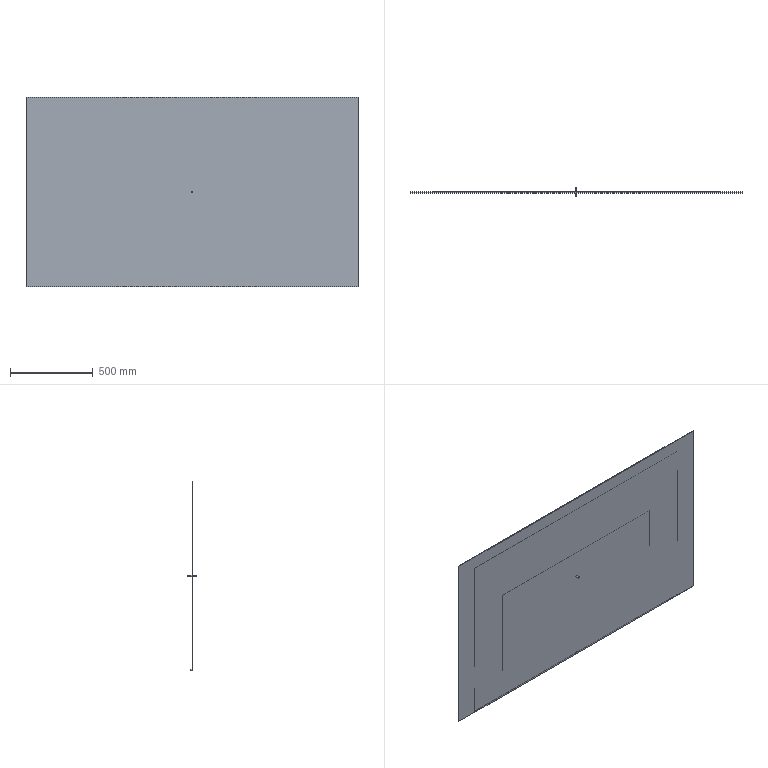Part | SolidWorks | features ICE 5, Extrusion 1 | 4 solids | 34 faces | box 2010 x 50 x 1150 mm | volume 11975475 mm3 | plane 28 | cylinder 6 | commonest cylinder face diameters 10 x6
STEP:
#1=CARTESIAN_POINT('',(1005.,-2.5,575.));
#2=VERTEX_POINT('',#1);
#3=CARTESIAN_POINT('',(1005.,-2.5,-575.));
#4=VERTEX_POINT('',#3);
#5=CARTESIAN_POINT('',(1005.,-2.5,575.));
#6=DIRECTION('',(0.,0.,-1.));
#7=VECTOR('',#6,1000.);
#8=LINE('',#5,#7);
#9=EDGE_CURVE('',#2,#4,#8,.T.);
#10=ORIENTED_EDGE('',*,*,#9,.T.);
#11=CARTESIAN_POINT('',(1005.,2.5,-575.));
#12=VERTEX_POINT('',#11);
#13=CARTESIAN_POINT('',(1005.,2.5,-575.));
#14=DIRECTION('',(0.,-1.,0.));
#15=VECTOR('',#14,1000.);
#16=LINE('',#13,#15);
#17=EDGE_CURVE('',#12,#4,#16,.T.);
#18=ORIENTED_EDGE('',*,*,#17,.F.);
#19=CARTESIAN_POINT('',(1005.,2.5,575.));
#20=VERTEX_POINT('',#19);
#21=CARTESIAN_POINT('',(1005.,2.5,575.));
#22=DIRECTION('',(0.,0.,-1.));
#23=VECTOR('',#22,1000.);
#24=LINE('',#21,#23);
#25=EDGE_CURVE('',#20,#12,#24,.T.);
#26=ORIENTED_EDGE('',*,*,#25,.F.);
#27=CARTESIAN_POINT('',(1005.,2.5,575.));
#28=DIRECTION('',(0.,-1.,0.));
#29=VECTOR('',#28,1000.);
#30=LINE('',#27,#29);
#31=EDGE_CURVE('',#20,#2,#30,.T.);
#32=ORIENTED_EDGE('',*,*,#31,.T.);
#33=EDGE_LOOP('',(#10,#18,#26,#32));
#34=FACE_OUTER_BOUND('',#33,.T.);
#35=CARTESIAN_POINT('',(1005.,2.5,575.));
#36=DIRECTION('',(-1.,0.,0.));
#37=DIRECTION('',(0.,0.,1.));
#38=AXIS2_PLACEMENT_3D('',#35,#36,#37);
#39=PLANE('',#38);
#40=ADVANCED_FACE('',(#34),#39,.F.);
#41=CARTESIAN_POINT('',(-1005.,-2.5,-575.));
#42=VERTEX_POINT('',#41);
#43=CARTESIAN_POINT('',(-1005.,-2.5,-575.));
#44=DIRECTION('',(-1.,0.,0.));
#45=VECTOR('',#44,1000.);
#46=LINE('',#43,#45);
#47=EDGE_CURVE('',#4,#42,#46,.T.);
#48=ORIENTED_EDGE('',*,*,#47,.T.);
#49=CARTESIAN_POINT('',(-1005.,2.5,-575.));
#50=VERTEX_POINT('',#49);
#51=CARTESIAN_POINT('',(-1005.,2.5,-575.));
#52=DIRECTION('',(0.,-1.,0.));
#53=VECTOR('',#52,1000.);
#54=LINE('',#51,#53);
#55=EDGE_CURVE('',#50,#42,#54,.T.);
#56=ORIENTED_EDGE('',*,*,#55,.F.);
#57=CARTESIAN_POINT('',(-1005.,2.5,-575.));
#58=DIRECTION('',(-1.,0.,0.));
#59=VECTOR('',#58,1000.);
#60=LINE('',#57,#59);
#61=EDGE_CURVE('',#12,#50,#60,.T.);
#62=ORIENTED_EDGE('',*,*,#61,.F.);
#63=ORIENTED_EDGE('',*,*,#17,.T.);
#64=EDGE_LOOP('',(#48,#56,#62,#63));
#65=FACE_OUTER_BOUND('',#64,.T.);
#66=CARTESIAN_POINT('',(-1005.,2.5,-575.));
#67=DIRECTION('',(0.,0.,1.));
#68=DIRECTION('',(1.,0.,0.));
#69=AXIS2_PLACEMENT_3D('',#66,#67,#68);
#70=PLANE('',#69);
#71=ADVANCED_FACE('',(#65),#70,.F.);
#72=CARTESIAN_POINT('',(-1005.,-2.5,575.));
#73=VERTEX_POINT('',#72);
#74=CARTESIAN_POINT('',(-1005.,-2.5,575.));
#75=DIRECTION('',(0.,0.,1.));
#76=VECTOR('',#75,1000.);
#77=LINE('',#74,#76);
#78=EDGE_CURVE('',#42,#73,#77,.T.);
#79=ORIENTED_EDGE('',*,*,#78,.T.);
#80=CARTESIAN_POINT('',(-1005.,2.5,575.));
#81=VERTEX_POINT('',#80);
#82=CARTESIAN_POINT('',(-1005.,2.5,575.));
#83=DIRECTION('',(0.,-1.,0.));
#84=VECTOR('',#83,1000.);
#85=LINE('',#82,#84);
#86=EDGE_CURVE('',#81,#73,#85,.T.);
#87=ORIENTED_EDGE('',*,*,#86,.F.);
#88=CARTESIAN_POINT('',(-1005.,2.5,575.));
#89=DIRECTION('',(0.,0.,1.));
#90=VECTOR('',#89,1000.);
#91=LINE('',#88,#90);
#92=EDGE_CURVE('',#50,#81,#91,.T.);
#93=ORIENTED_EDGE('',*,*,#92,.F.);
#94=ORIENTED_EDGE('',*,*,#55,.T.);
#95=EDGE_LOOP('',(#79,#87,#93,#94));
#96=FACE_OUTER_BOUND('',#95,.T.);
#97=CARTESIAN_POINT('',(-1005.,2.5,575.));
#98=DIRECTION('',(1.,0.,0.));
#99=DIRECTION('',(0.,0.,-1.));
#100=AXIS2_PLACEMENT_3D('',#97,#98,#99);
#101=PLANE('',#100);
#102=ADVANCED_FACE('',(#96),#101,.F.);
#103=CARTESIAN_POINT('',(-1005.,-2.5,575.));
#104=DIRECTION('',(1.,0.,0.));
#105=VECTOR('',#104,1000.);
#106=LINE('',#103,#105);
#107=EDGE_CURVE('',#73,#2,#106,.T.);
#108=ORIENTED_EDGE('',*,*,#107,.T.);
#109=ORIENTED_EDGE('',*,*,#31,.F.);
#110=CARTESIAN_POINT('',(-1005.,2.5,575.));
#111=DIRECTION('',(1.,0.,0.));
#112=VECTOR('',#111,1000.);
#113=LINE('',#110,#112);
#114=EDGE_CURVE('',#81,#20,#113,.T.);
#115=ORIENTED_EDGE('',*,*,#114,.F.);
#116=ORIENTED_EDGE('',*,*,#86,.T.);
#117=EDGE_LOOP('',(#108,#109,#115,#116));
#118=FACE_OUTER_BOUND('',#117,.T.);
#119=CARTESIAN_POINT('',(-1005.,2.5,575.));
#120=DIRECTION('',(0.,0.,-1.));
#121=DIRECTION('',(-1.,0.,0.));
#122=AXIS2_PLACEMENT_3D('',#119,#120,#121);
#123=PLANE('',#122);
#124=ADVANCED_FACE('',(#118),#123,.F.);
#125=ORIENTED_EDGE('',*,*,#25,.T.);
#126=ORIENTED_EDGE('',*,*,#61,.T.);
#127=ORIENTED_EDGE('',*,*,#92,.T.);
#128=ORIENTED_EDGE('',*,*,#114,.T.);
#129=EDGE_LOOP('',(#125,#126,#127,#128));
#130=FACE_OUTER_BOUND('',#129,.T.);
#131=CARTESIAN_POINT('',(0.,2.5,0.));
#132=DIRECTION('',(0.,-1.,0.));
#133=DIRECTION('',(0.,0.,-1.));
#134=AXIS2_PLACEMENT_3D('',#131,#132,#133);
#135=PLANE('',#134);
#136=ADVANCED_FACE('',(#130),#135,.F.);
#137=ORIENTED_EDGE('',*,*,#9,.F.);
#138=ORIENTED_EDGE('',*,*,#107,.F.);
#139=ORIENTED_EDGE('',*,*,#78,.F.);
#140=ORIENTED_EDGE('',*,*,#47,.F.);
#141=EDGE_LOOP('',(#137,#138,#139,#140));
#142=FACE_OUTER_BOUND('',#141,.T.);
#143=CARTESIAN_POINT('',(0.,-2.5,0.));
#144=DIRECTION('',(0.,-1.,0.));
#145=DIRECTION('',(0.,0.,-1.));
#146=AXIS2_PLACEMENT_3D('',#143,#144,#145);
#147=PLANE('',#146);
#148=ADVANCED_FACE('',(#142),#147,.T.);
#149=CLOSED_SHELL('',(#40,#71,#102,#124,#136,#148));
#150=MANIFOLD_SOLID_BREP('',#149);
#151=CARTESIAN_POINT('',(870.,2.6,491.5));
#152=VERTEX_POINT('',#151);
#153=CARTESIAN_POINT('',(870.,2.6,-568.5));
#154=VERTEX_POINT('',#153);
#155=CARTESIAN_POINT('',(870.,2.6,491.5));
#156=DIRECTION('',(0.,0.,-1.));
#157=VECTOR('',#156,1000.);
#158=LINE('',#155,#157);
#159=EDGE_CURVE('',#152,#154,#158,.T.);
#160=ORIENTED_EDGE('',*,*,#159,.T.);
#161=CARTESIAN_POINT('',(870.,2.7,-568.5));
#162=VERTEX_POINT('',#161);
#163=CARTESIAN_POINT('',(870.,2.7,-568.5));
#164=DIRECTION('',(0.,-1.,0.));
#165=VECTOR('',#164,1000.);
#166=LINE('',#163,#165);
#167=EDGE_CURVE('',#162,#154,#166,.T.);
#168=ORIENTED_EDGE('',*,*,#167,.F.);
#169=CARTESIAN_POINT('',(870.,2.7,491.5));
#170=VERTEX_POINT('',#169);
#171=CARTESIAN_POINT('',(870.,2.7,491.5));
#172=DIRECTION('',(0.,0.,-1.));
#173=VECTOR('',#172,1000.);
#174=LINE('',#171,#173);
#175=EDGE_CURVE('',#170,#162,#174,.T.);
#176=ORIENTED_EDGE('',*,*,#175,.F.);
#177=CARTESIAN_POINT('',(870.,2.7,491.5));
#178=DIRECTION('',(0.,-1.,0.));
#179=VECTOR('',#178,1000.);
#180=LINE('',#177,#179);
#181=EDGE_CURVE('',#170,#152,#180,.T.);
#182=ORIENTED_EDGE('',*,*,#181,.T.);
#183=EDGE_LOOP('',(#160,#168,#176,#182));
#184=FACE_OUTER_BOUND('',#183,.T.);
#185=CARTESIAN_POINT('',(870.,2.7,491.5));
#186=DIRECTION('',(-1.,0.,0.));
#187=DIRECTION('',(0.,0.,1.));
#188=AXIS2_PLACEMENT_3D('',#185,#186,#187);
#189=PLANE('',#188);
#190=ADVANCED_FACE('',(#184),#189,.F.);
#191=CARTESIAN_POINT('',(-870.,2.6,-568.5));
#192=VERTEX_POINT('',#191);
#193=CARTESIAN_POINT('',(-870.,2.6,-568.5));
#194=DIRECTION('',(-1.,0.,0.));
#195=VECTOR('',#194,1000.);
#196=LINE('',#193,#195);
#197=EDGE_CURVE('',#154,#192,#196,.T.);
#198=ORIENTED_EDGE('',*,*,#197,.T.);
#199=CARTESIAN_POINT('',(-870.,2.7,-568.5));
#200=VERTEX_POINT('',#199);
#201=CARTESIAN_POINT('',(-870.,2.7,-568.5));
#202=DIRECTION('',(0.,-1.,0.));
#203=VECTOR('',#202,1000.);
#204=LINE('',#201,#203);
#205=EDGE_CURVE('',#200,#192,#204,.T.);
#206=ORIENTED_EDGE('',*,*,#205,.F.);
#207=CARTESIAN_POINT('',(-870.,2.7,-568.5));
#208=DIRECTION('',(-1.,0.,0.));
#209=VECTOR('',#208,1000.);
#210=LINE('',#207,#209);
#211=EDGE_CURVE('',#162,#200,#210,.T.);
#212=ORIENTED_EDGE('',*,*,#211,.F.);
#213=ORIENTED_EDGE('',*,*,#167,.T.);
#214=EDGE_LOOP('',(#198,#206,#212,#213));
#215=FACE_OUTER_BOUND('',#214,.T.);
#216=CARTESIAN_POINT('',(-870.,2.7,-568.5));
#217=DIRECTION('',(0.,0.,1.));
#218=DIRECTION('',(1.,0.,0.));
#219=AXIS2_PLACEMENT_3D('',#216,#217,#218);
#220=PLANE('',#219);
#221=ADVANCED_FACE('',(#215),#220,.F.);
#222=CARTESIAN_POINT('',(-870.,2.6,491.5));
#223=VERTEX_POINT('',#222);
#224=CARTESIAN_POINT('',(-870.,2.6,491.5));
#225=DIRECTION('',(0.,0.,1.));
#226=VECTOR('',#225,1000.);
#227=LINE('',#224,#226);
#228=EDGE_CURVE('',#192,#223,#227,.T.);
#229=ORIENTED_EDGE('',*,*,#228,.T.);
#230=CARTESIAN_POINT('',(-870.,2.7,491.5));
#231=VERTEX_POINT('',#230);
#232=CARTESIAN_POINT('',(-870.,2.7,491.5));
#233=DIRECTION('',(0.,-1.,0.));
#234=VECTOR('',#233,1000.);
#235=LINE('',#232,#234);
#236=EDGE_CURVE('',#231,#223,#235,.T.);
#237=ORIENTED_EDGE('',*,*,#236,.F.);
#238=CARTESIAN_POINT('',(-870.,2.7,491.5));
#239=DIRECTION('',(0.,0.,1.));
#240=VECTOR('',#239,1000.);
#241=LINE('',#238,#240);
#242=EDGE_CURVE('',#200,#231,#241,.T.);
#243=ORIENTED_EDGE('',*,*,#242,.F.);
#244=ORIENTED_EDGE('',*,*,#205,.T.);
#245=EDGE_LOOP('',(#229,#237,#243,#244));
#246=FACE_OUTER_BOUND('',#245,.T.);
#247=CARTESIAN_POINT('',(-870.,2.7,491.5));
#248=DIRECTION('',(1.,0.,0.));
#249=DIRECTION('',(0.,0.,-1.));
#250=AXIS2_PLACEMENT_3D('',#247,#248,#249);
#251=PLANE('',#250);
#252=ADVANCED_FACE('',(#246),#251,.F.);
#253=CARTESIAN_POINT('',(-870.,2.6,491.5));
#254=DIRECTION('',(1.,0.,0.));
#255=VECTOR('',#254,1000.);
#256=LINE('',#253,#255);
#257=EDGE_CURVE('',#223,#152,#256,.T.);
#258=ORIENTED_EDGE('',*,*,#257,.T.);
#259=ORIENTED_EDGE('',*,*,#181,.F.);
#260=CARTESIAN_POINT('',(-870.,2.7,491.5));
#261=DIRECTION('',(1.,0.,0.));
#262=VECTOR('',#261,1000.);
#263=LINE('',#260,#262);
#264=EDGE_CURVE('',#231,#170,#263,.T.);
#265=ORIENTED_EDGE('',*,*,#264,.F.);
#266=ORIENTED_EDGE('',*,*,#236,.T.);
#267=EDGE_LOOP('',(#258,#259,#265,#266));
#268=FACE_OUTER_BOUND('',#267,.T.);
#269=CARTESIAN_POINT('',(-870.,2.7,491.5));
#270=DIRECTION('',(0.,0.,-1.));
#271=DIRECTION('',(-1.,0.,0.));
#272=AXIS2_PLACEMENT_3D('',#269,#270,#271);
#273=PLANE('',#272);
#274=ADVANCED_FACE('',(#268),#273,.F.);
#275=ORIENTED_EDGE('',*,*,#175,.T.);
#276=ORIENTED_EDGE('',*,*,#211,.T.);
#277=ORIENTED_EDGE('',*,*,#242,.T.);
#278=ORIENTED_EDGE('',*,*,#264,.T.);
#279=EDGE_LOOP('',(#275,#276,#277,#278));
#280=FACE_OUTER_BOUND('',#279,.T.);
#281=CARTESIAN_POINT('',(0.,2.7,0.));
#282=DIRECTION('',(0.,-1.,0.));
#283=DIRECTION('',(0.,0.,-1.));
#284=AXIS2_PLACEMENT_3D('',#281,#282,#283);
#285=PLANE('',#284);
#286=ADVANCED_FACE('',(#280),#285,.F.);
#287=ORIENTED_EDGE('',*,*,#159,.F.);
#288=ORIENTED_EDGE('',*,*,#257,.F.);
#289=ORIENTED_EDGE('',*,*,#228,.F.);
#290=ORIENTED_EDGE('',*,*,#197,.F.);
#291=EDGE_LOOP('',(#287,#288,#289,#290));
#292=FACE_OUTER_BOUND('',#291,.T.);
#293=CARTESIAN_POINT('',(0.,2.6,0.));
#294=DIRECTION('',(0.,-1.,0.));
#295=DIRECTION('',(0.,0.,-1.));
#296=AXIS2_PLACEMENT_3D('',#293,#294,#295);
#297=PLANE('',#296);
#298=ADVANCED_FACE('',(#292),#297,.T.);
#299=CLOSED_SHELL('',(#190,#221,#252,#274,#286,#298));
#300=MANIFOLD_SOLID_BREP('',#299);
#301=CARTESIAN_POINT('',(745.,2.7,341.5));
#302=VERTEX_POINT('',#301);
#303=CARTESIAN_POINT('',(745.,2.7,-568.5));
#304=VERTEX_POINT('',#303);
#305=CARTESIAN_POINT('',(745.,2.7,341.5));
#306=DIRECTION('',(0.,0.,-1.));
#307=VECTOR('',#306,1000.);
#308=LINE('',#305,#307);
#309=EDGE_CURVE('',#302,#304,#308,.T.);
#310=ORIENTED_EDGE('',*,*,#309,.T.);
#311=CARTESIAN_POINT('',(745.,2.8,-568.5));
#312=VERTEX_POINT('',#311);
#313=CARTESIAN_POINT('',(745.,2.8,-568.5));
#314=DIRECTION('',(0.,-1.,0.));
#315=VECTOR('',#314,1000.);
#316=LINE('',#313,#315);
#317=EDGE_CURVE('',#312,#304,#316,.T.);
#318=ORIENTED_EDGE('',*,*,#317,.F.);
#319=CARTESIAN_POINT('',(745.,2.8,341.5));
#320=VERTEX_POINT('',#319);
#321=CARTESIAN_POINT('',(745.,2.8,341.5));
#322=DIRECTION('',(0.,0.,-1.));
#323=VECTOR('',#322,1000.);
#324=LINE('',#321,#323);
#325=EDGE_CURVE('',#320,#312,#324,.T.);
#326=ORIENTED_EDGE('',*,*,#325,.F.);
#327=CARTESIAN_POINT('',(745.,2.8,341.5));
#328=DIRECTION('',(0.,-1.,0.));
#329=VECTOR('',#328,1000.);
#330=LINE('',#327,#329);
#331=EDGE_CURVE('',#320,#302,#330,.T.);
#332=ORIENTED_EDGE('',*,*,#331,.T.);
#333=EDGE_LOOP('',(#310,#318,#326,#332));
#334=FACE_OUTER_BOUND('',#333,.T.);
#335=CARTESIAN_POINT('',(745.,2.8,341.5));
#336=DIRECTION('',(-1.,0.,0.));
#337=DIRECTION('',(0.,0.,1.));
#338=AXIS2_PLACEMENT_3D('',#335,#336,#337);
#339=PLANE('',#338);
#340=ADVANCED_FACE('',(#334),#339,.F.);
#341=CARTESIAN_POINT('',(-745.,2.7,-568.5));
#342=VERTEX_POINT('',#341);
#343=CARTESIAN_POINT('',(-745.,2.7,-568.5));
#344=DIRECTION('',(-1.,0.,0.));
#345=VECTOR('',#344,1000.);
#346=LINE('',#343,#345);
#347=EDGE_CURVE('',#304,#342,#346,.T.);
#348=ORIENTED_EDGE('',*,*,#347,.T.);
#349=CARTESIAN_POINT('',(-745.,2.8,-568.5));
#350=VERTEX_POINT('',#349);
#351=CARTESIAN_POINT('',(-745.,2.8,-568.5));
#352=DIRECTION('',(0.,-1.,0.));
#353=VECTOR('',#352,1000.);
#354=LINE('',#351,#353);
#355=EDGE_CURVE('',#350,#342,#354,.T.);
#356=ORIENTED_EDGE('',*,*,#355,.F.);
#357=CARTESIAN_POINT('',(-745.,2.8,-568.5));
#358=DIRECTION('',(-1.,0.,0.));
#359=VECTOR('',#358,1000.);
#360=LINE('',#357,#359);
#361=EDGE_CURVE('',#312,#350,#360,.T.);
#362=ORIENTED_EDGE('',*,*,#361,.F.);
#363=ORIENTED_EDGE('',*,*,#317,.T.);
#364=EDGE_LOOP('',(#348,#356,#362,#363));
#365=FACE_OUTER_BOUND('',#364,.T.);
#366=CARTESIAN_POINT('',(-745.,2.8,-568.5));
#367=DIRECTION('',(0.,0.,1.));
#368=DIRECTION('',(1.,0.,0.));
#369=AXIS2_PLACEMENT_3D('',#366,#367,#368);
#370=PLANE('',#369);
#371=ADVANCED_FACE('',(#365),#370,.F.);
#372=CARTESIAN_POINT('',(-745.,2.7,341.5));
#373=VERTEX_POINT('',#372);
#374=CARTESIAN_POINT('',(-745.,2.7,341.5));
#375=DIRECTION('',(0.,0.,1.));
#376=VECTOR('',#375,1000.);
#377=LINE('',#374,#376);
#378=EDGE_CURVE('',#342,#373,#377,.T.);
#379=ORIENTED_EDGE('',*,*,#378,.T.);
#380=CARTESIAN_POINT('',(-745.,2.8,341.5));
#381=VERTEX_POINT('',#380);
#382=CARTESIAN_POINT('',(-745.,2.8,341.5));
#383=DIRECTION('',(0.,-1.,0.));
#384=VECTOR('',#383,1000.);
#385=LINE('',#382,#384);
#386=EDGE_CURVE('',#381,#373,#385,.T.);
#387=ORIENTED_EDGE('',*,*,#386,.F.);
#388=CARTESIAN_POINT('',(-745.,2.8,341.5));
#389=DIRECTION('',(0.,0.,1.));
#390=VECTOR('',#389,1000.);
#391=LINE('',#388,#390);
#392=EDGE_CURVE('',#350,#381,#391,.T.);
#393=ORIENTED_EDGE('',*,*,#392,.F.);
#394=ORIENTED_EDGE('',*,*,#355,.T.);
#395=EDGE_LOOP('',(#379,#387,#393,#394));
#396=FACE_OUTER_BOUND('',#395,.T.);
#397=CARTESIAN_POINT('',(-745.,2.8,341.5));
#398=DIRECTION('',(1.,0.,0.));
#399=DIRECTION('',(0.,0.,-1.));
#400=AXIS2_PLACEMENT_3D('',#397,#398,#399);
#401=PLANE('',#400);
#402=ADVANCED_FACE('',(#396),#401,.F.);
#403=CARTESIAN_POINT('',(-745.,2.7,341.5));
#404=DIRECTION('',(1.,0.,0.));
#405=VECTOR('',#404,1000.);
#406=LINE('',#403,#405);
#407=EDGE_CURVE('',#373,#302,#406,.T.);
#408=ORIENTED_EDGE('',*,*,#407,.T.);
#409=ORIENTED_EDGE('',*,*,#331,.F.);
#410=CARTESIAN_POINT('',(-745.,2.8,341.5));
#411=DIRECTION('',(1.,0.,0.));
#412=VECTOR('',#411,1000.);
#413=LINE('',#410,#412);
#414=EDGE_CURVE('',#381,#320,#413,.T.);
#415=ORIENTED_EDGE('',*,*,#414,.F.);
#416=ORIENTED_EDGE('',*,*,#386,.T.);
#417=EDGE_LOOP('',(#408,#409,#415,#416));
#418=FACE_OUTER_BOUND('',#417,.T.);
#419=CARTESIAN_POINT('',(-745.,2.8,341.5));
#420=DIRECTION('',(0.,0.,-1.));
#421=DIRECTION('',(-1.,0.,0.));
#422=AXIS2_PLACEMENT_3D('',#419,#420,#421);
#423=PLANE('',#422);
#424=ADVANCED_FACE('',(#418),#423,.F.);
#425=ORIENTED_EDGE('',*,*,#325,.T.);
#426=ORIENTED_EDGE('',*,*,#361,.T.);
#427=ORIENTED_EDGE('',*,*,#392,.T.);
#428=ORIENTED_EDGE('',*,*,#414,.T.);
#429=EDGE_LOOP('',(#425,#426,#427,#428));
#430=FACE_OUTER_BOUND('',#429,.T.);
#431=CARTESIAN_POINT('',(0.,2.8,0.));
#432=DIRECTION('',(0.,-1.,0.));
#433=DIRECTION('',(0.,0.,-1.));
#434=AXIS2_PLACEMENT_3D('',#431,#432,#433);
#435=PLANE('',#434);
#436=ADVANCED_FACE('',(#430),#435,.F.);
#437=ORIENTED_EDGE('',*,*,#309,.F.);
#438=ORIENTED_EDGE('',*,*,#407,.F.);
#439=ORIENTED_EDGE('',*,*,#378,.F.);
#440=ORIENTED_EDGE('',*,*,#347,.F.);
#441=EDGE_LOOP('',(#437,#438,#439,#440));
#442=FACE_OUTER_BOUND('',#441,.T.);
#443=CARTESIAN_POINT('',(0.,2.7,0.));
#444=DIRECTION('',(0.,-1.,0.));
#445=DIRECTION('',(0.,0.,-1.));
#446=AXIS2_PLACEMENT_3D('',#443,#444,#445);
#447=PLANE('',#446);
#448=ADVANCED_FACE('',(#442),#447,.T.);
#449=CLOSED_SHELL('',(#340,#371,#402,#424,#436,#448));
#450=MANIFOLD_SOLID_BREP('',#449);
#451=CARTESIAN_POINT('',(0.,12.9,-563.5));
#452=VERTEX_POINT('',#451);
#453=CARTESIAN_POINT('',(0.,12.9,-573.5));
#454=VERTEX_POINT('',#453);
#455=CARTESIAN_POINT('',(0.,12.9,-568.5));
#456=DIRECTION('',(0.,1.,0.));
#457=DIRECTION('',(0.,0.,1.));
#458=AXIS2_PLACEMENT_3D('',#455,#456,#457);
#459=CIRCLE('',#458,5.);
#460=EDGE_CURVE('',#452,#454,#459,.T.);
#461=ORIENTED_EDGE('',*,*,#460,.F.);
#462=CARTESIAN_POINT('',(0.,2.9,-563.5));
#463=VERTEX_POINT('',#462);
#464=CARTESIAN_POINT('',(0.,12.9,-563.5));
#465=DIRECTION('',(0.,-1.,0.));
#466=VECTOR('',#465,1000.);
#467=LINE('',#464,#466);
#468=EDGE_CURVE('',#452,#463,#467,.T.);
#469=ORIENTED_EDGE('',*,*,#468,.T.);
#470=CARTESIAN_POINT('',(5.,2.9,-568.5));
#471=VERTEX_POINT('',#470);
#472=CARTESIAN_POINT('',(0.,2.9,-568.5));
#473=DIRECTION('',(0.,1.,0.));
#474=DIRECTION('',(0.,0.,1.));
#475=AXIS2_PLACEMENT_3D('',#472,#473,#474);
#476=CIRCLE('',#475,5.);
#477=EDGE_CURVE('',#463,#471,#476,.T.);
#478=ORIENTED_EDGE('',*,*,#477,.T.);
#479=CARTESIAN_POINT('',(0.,2.9,-573.5));
#480=VERTEX_POINT('',#479);
#481=CARTESIAN_POINT('',(0.,2.9,-568.5));
#482=DIRECTION('',(0.,1.,0.));
#483=DIRECTION('',(0.,0.,1.));
#484=AXIS2_PLACEMENT_3D('',#481,#482,#483);
#485=CIRCLE('',#484,5.);
#486=EDGE_CURVE('',#471,#480,#485,.T.);
#487=ORIENTED_EDGE('',*,*,#486,.T.);
#488=CARTESIAN_POINT('',(0.,12.9,-573.5));
#489=DIRECTION('',(0.,-1.,0.));
#490=VECTOR('',#489,1000.);
#491=LINE('',#488,#490);
#492=EDGE_CURVE('',#454,#480,#491,.T.);
#493=ORIENTED_EDGE('',*,*,#492,.F.);
#494=EDGE_LOOP('',(#461,#469,#478,#487,#493));
#495=FACE_OUTER_BOUND('',#494,.T.);
#496=CARTESIAN_POINT('',(0.,12.9,-568.5));
#497=DIRECTION('',(0.,-1.,0.));
#498=DIRECTION('',(0.,0.,-1.));
#499=AXIS2_PLACEMENT_3D('',#496,#497,#498);
#500=CYLINDRICAL_SURFACE('',#499,5.);
#501=ADVANCED_FACE('',(#495),#500,.T.);
#502=CARTESIAN_POINT('',(0.,27.9,5.));
#503=VERTEX_POINT('',#502);
#504=CARTESIAN_POINT('',(0.,27.9,-5.));
#505=VERTEX_POINT('',#504);
#506=CARTESIAN_POINT('',(0.,27.9,0.));
#507=DIRECTION('',(0.,1.,0.));
#508=DIRECTION('',(0.,0.,1.));
#509=AXIS2_PLACEMENT_3D('',#506,#507,#508);
#510=CIRCLE('',#509,5.);
#511=EDGE_CURVE('',#503,#505,#510,.T.);
#512=ORIENTED_EDGE('',*,*,#511,.F.);
#513=CARTESIAN_POINT('',(0.,2.9,5.));
#514=VERTEX_POINT('',#513);
#515=CARTESIAN_POINT('',(0.,27.9,5.));
#516=DIRECTION('',(0.,-1.,0.));
#517=VECTOR('',#516,1000.);
#518=LINE('',#515,#517);
#519=EDGE_CURVE('',#503,#514,#518,.T.);
#520=ORIENTED_EDGE('',*,*,#519,.T.);
#521=CARTESIAN_POINT('',(0.,2.9,-5.));
#522=VERTEX_POINT('',#521);
#523=CARTESIAN_POINT('',(0.,2.9,0.));
#524=DIRECTION('',(0.,1.,0.));
#525=DIRECTION('',(0.,0.,-1.));
#526=AXIS2_PLACEMENT_3D('',#523,#524,#525);
#527=CIRCLE('',#526,5.);
#528=EDGE_CURVE('',#514,#522,#527,.T.);
#529=ORIENTED_EDGE('',*,*,#528,.T.);
#530=CARTESIAN_POINT('',(0.,27.9,-5.));
#531=DIRECTION('',(0.,-1.,0.));
#532=VECTOR('',#531,1000.);
#533=LINE('',#530,#532);
#534=EDGE_CURVE('',#505,#522,#533,.T.);
#535=ORIENTED_EDGE('',*,*,#534,.F.);
#536=EDGE_LOOP('',(#512,#520,#529,#535));
#537=FACE_OUTER_BOUND('',#536,.T.);
#538=CARTESIAN_POINT('',(0.,27.9,0.));
#539=DIRECTION('',(0.,-1.,0.));
#540=DIRECTION('',(0.,0.,-1.));
#541=AXIS2_PLACEMENT_3D('',#538,#539,#540);
#542=CYLINDRICAL_SURFACE('',#541,5.);
#543=ADVANCED_FACE('',(#537),#542,.T.);
#544=CARTESIAN_POINT('',(0.,2.8,5.));
#545=VERTEX_POINT('',#544);
#546=CARTESIAN_POINT('',(0.,2.8,-5.));
#547=VERTEX_POINT('',#546);
#548=CARTESIAN_POINT('',(0.,2.8,0.));
#549=DIRECTION('',(0.,1.,0.));
#550=DIRECTION('',(0.,0.,-1.));
#551=AXIS2_PLACEMENT_3D('',#548,#549,#550);
#552=CIRCLE('',#551,5.);
#553=EDGE_CURVE('',#545,#547,#552,.T.);
#554=ORIENTED_EDGE('',*,*,#553,.F.);
#555=CARTESIAN_POINT('',(0.,-22.1,5.));
#556=VERTEX_POINT('',#555);
#557=CARTESIAN_POINT('',(0.,27.9,5.));
#558=DIRECTION('',(0.,-1.,0.));
#559=VECTOR('',#558,1000.);
#560=LINE('',#557,#559);
#561=EDGE_CURVE('',#545,#556,#560,.T.);
#562=ORIENTED_EDGE('',*,*,#561,.T.);
#563=CARTESIAN_POINT('',(0.,-22.1,-5.));
#564=VERTEX_POINT('',#563);
#565=CARTESIAN_POINT('',(0.,-22.1,0.));
#566=DIRECTION('',(0.,1.,0.));
#567=DIRECTION('',(0.,0.,1.));
#568=AXIS2_PLACEMENT_3D('',#565,#566,#567);
#569=CIRCLE('',#568,5.);
#570=EDGE_CURVE('',#556,#564,#569,.T.);
#571=ORIENTED_EDGE('',*,*,#570,.T.);
#572=CARTESIAN_POINT('',(0.,27.9,-5.));
#573=DIRECTION('',(0.,-1.,0.));
#574=VECTOR('',#573,1000.);
#575=LINE('',#572,#574);
#576=EDGE_CURVE('',#547,#564,#575,.T.);
#577=ORIENTED_EDGE('',*,*,#576,.F.);
#578=EDGE_LOOP('',(#554,#562,#571,#577));
#579=FACE_OUTER_BOUND('',#578,.T.);
#580=CARTESIAN_POINT('',(0.,27.9,0.));
#581=DIRECTION('',(0.,-1.,0.));
#582=DIRECTION('',(0.,0.,-1.));
#583=AXIS2_PLACEMENT_3D('',#580,#581,#582);
#584=CYLINDRICAL_SURFACE('',#583,5.);
#585=ADVANCED_FACE('',(#579),#584,.T.);
#586=CARTESIAN_POINT('',(-5.,2.9,-568.5));
#587=VERTEX_POINT('',#586);
#588=CARTESIAN_POINT('',(0.,2.9,-568.5));
#589=DIRECTION('',(0.,1.,0.));
#590=DIRECTION('',(0.,0.,1.));
#591=AXIS2_PLACEMENT_3D('',#588,#589,#590);
#592=CIRCLE('',#591,5.);
#593=EDGE_CURVE('',#587,#463,#592,.T.);
#594=ORIENTED_EDGE('',*,*,#593,.F.);
#595=CARTESIAN_POINT('',(-630.,2.9,-568.5));
#596=VERTEX_POINT('',#595);
#597=CARTESIAN_POINT('',(-630.,2.9,-568.5));
#598=DIRECTION('',(-1.,0.,0.));
#599=VECTOR('',#598,1000.);
#600=LINE('',#597,#599);
#601=EDGE_CURVE('',#587,#596,#600,.T.);
#602=ORIENTED_EDGE('',*,*,#601,.T.);
#603=CARTESIAN_POINT('',(-630.,2.9,171.5));
#604=VERTEX_POINT('',#603);
#605=CARTESIAN_POINT('',(-630.,2.9,171.5));
#606=DIRECTION('',(0.,0.,1.));
#607=VECTOR('',#606,1000.);
#608=LINE('',#605,#607);
#609=EDGE_CURVE('',#596,#604,#608,.T.);
#610=ORIENTED_EDGE('',*,*,#609,.T.);
#611=CARTESIAN_POINT('',(630.,2.9,171.5));
#612=VERTEX_POINT('',#611);
#613=CARTESIAN_POINT('',(-630.,2.9,171.5));
#614=DIRECTION('',(1.,0.,0.));
#615=VECTOR('',#614,1000.);
#616=LINE('',#613,#615);
#617=EDGE_CURVE('',#604,#612,#616,.T.);
#618=ORIENTED_EDGE('',*,*,#617,.T.);
#619=CARTESIAN_POINT('',(630.,2.9,-568.5));
#620=VERTEX_POINT('',#619);
#621=CARTESIAN_POINT('',(630.,2.9,171.5));
#622=DIRECTION('',(0.,0.,-1.));
#623=VECTOR('',#622,1000.);
#624=LINE('',#621,#623);
#625=EDGE_CURVE('',#612,#620,#624,.T.);
#626=ORIENTED_EDGE('',*,*,#625,.T.);
#627=CARTESIAN_POINT('',(-630.,2.9,-568.5));
#628=DIRECTION('',(-1.,0.,0.));
#629=VECTOR('',#628,1000.);
#630=LINE('',#627,#629);
#631=EDGE_CURVE('',#620,#471,#630,.T.);
#632=ORIENTED_EDGE('',*,*,#631,.T.);
#633=ORIENTED_EDGE('',*,*,#477,.F.);
#634=EDGE_LOOP('',(#594,#602,#610,#618,#626,#632,#633));
#635=FACE_OUTER_BOUND('',#634,.T.);
#636=CARTESIAN_POINT('',(0.,2.9,0.));
#637=DIRECTION('',(0.,1.,0.));
#638=DIRECTION('',(0.,0.,-1.));
#639=AXIS2_PLACEMENT_3D('',#636,#637,#638);
#640=CIRCLE('',#639,5.);
#641=EDGE_CURVE('',#522,#514,#640,.T.);
#642=ORIENTED_EDGE('',*,*,#641,.F.);
#643=ORIENTED_EDGE('',*,*,#528,.F.);
#644=EDGE_LOOP('',(#642,#643));
#645=FACE_BOUND('',#644,.T.);
#646=CARTESIAN_POINT('',(0.,2.9,0.));
#647=DIRECTION('',(0.,-1.,0.));
#648=DIRECTION('',(0.,0.,-1.));
#649=AXIS2_PLACEMENT_3D('',#646,#647,#648);
#650=PLANE('',#649);
#651=ADVANCED_FACE('',(#635,#645),#650,.F.);
#652=CARTESIAN_POINT('',(630.,2.8,171.5));
#653=VERTEX_POINT('',#652);
#654=CARTESIAN_POINT('',(630.,2.8,-568.5));
#655=VERTEX_POINT('',#654);
#656=CARTESIAN_POINT('',(630.,2.8,171.5));
#657=DIRECTION('',(0.,0.,-1.));
#658=VECTOR('',#657,1000.);
#659=LINE('',#656,#658);
#660=EDGE_CURVE('',#653,#655,#659,.T.);
#661=ORIENTED_EDGE('',*,*,#660,.F.);
#662=CARTESIAN_POINT('',(-630.,2.8,171.5));
#663=VERTEX_POINT('',#662);
#664=CARTESIAN_POINT('',(-630.,2.8,171.5));
#665=DIRECTION('',(1.,0.,0.));
#666=VECTOR('',#665,1000.);
#667=LINE('',#664,#666);
#668=EDGE_CURVE('',#663,#653,#667,.T.);
#669=ORIENTED_EDGE('',*,*,#668,.F.);
#670=CARTESIAN_POINT('',(-630.,2.8,-568.5));
#671=VERTEX_POINT('',#670);
#672=CARTESIAN_POINT('',(-630.,2.8,171.5));
#673=DIRECTION('',(0.,0.,1.));
#674=VECTOR('',#673,1000.);
#675=LINE('',#672,#674);
#676=EDGE_CURVE('',#671,#663,#675,.T.);
#677=ORIENTED_EDGE('',*,*,#676,.F.);
#678=CARTESIAN_POINT('',(-630.,2.8,-568.5));
#679=DIRECTION('',(-1.,0.,0.));
#680=VECTOR('',#679,1000.);
#681=LINE('',#678,#680);
#682=EDGE_CURVE('',#655,#671,#681,.T.);
#683=ORIENTED_EDGE('',*,*,#682,.F.);
#684=EDGE_LOOP('',(#661,#669,#677,#683));
#685=FACE_OUTER_BOUND('',#684,.T.);
#686=CARTESIAN_POINT('',(0.,2.8,0.));
#687=DIRECTION('',(0.,1.,0.));
#688=DIRECTION('',(0.,0.,-1.));
#689=AXIS2_PLACEMENT_3D('',#686,#687,#688);
#690=CIRCLE('',#689,5.);
#691=EDGE_CURVE('',#547,#545,#690,.T.);
#692=ORIENTED_EDGE('',*,*,#691,.T.);
#693=ORIENTED_EDGE('',*,*,#553,.T.);
#694=EDGE_LOOP('',(#692,#693));
#695=FACE_BOUND('',#694,.T.);
#696=CARTESIAN_POINT('',(0.,2.8,0.));
#697=DIRECTION('',(0.,-1.,0.));
#698=DIRECTION('',(0.,0.,-1.));
#699=AXIS2_PLACEMENT_3D('',#696,#697,#698);
#700=PLANE('',#699);
#701=ADVANCED_FACE('',(#685,#695),#700,.T.);
#702=ORIENTED_EDGE('',*,*,#660,.T.);
#703=CARTESIAN_POINT('',(630.,2.9,-568.5));
#704=DIRECTION('',(0.,-1.,0.));
#705=VECTOR('',#704,1000.);
#706=LINE('',#703,#705);
#707=EDGE_CURVE('',#620,#655,#706,.T.);
#708=ORIENTED_EDGE('',*,*,#707,.F.);
#709=ORIENTED_EDGE('',*,*,#625,.F.);
#710=CARTESIAN_POINT('',(630.,2.9,171.5));
#711=DIRECTION('',(0.,-1.,0.));
#712=VECTOR('',#711,1000.);
#713=LINE('',#710,#712);
#714=EDGE_CURVE('',#612,#653,#713,.T.);
#715=ORIENTED_EDGE('',*,*,#714,.T.);
#716=EDGE_LOOP('',(#702,#708,#709,#715));
#717=FACE_OUTER_BOUND('',#716,.T.);
#718=CARTESIAN_POINT('',(630.,2.9,171.5));
#719=DIRECTION('',(-1.,0.,0.));
#720=DIRECTION('',(0.,0.,1.));
#721=AXIS2_PLACEMENT_3D('',#718,#719,#720);
#722=PLANE('',#721);
#723=ADVANCED_FACE('',(#717),#722,.F.);
#724=ORIENTED_EDGE('',*,*,#682,.T.);
#725=CARTESIAN_POINT('',(-630.,2.9,-568.5));
#726=DIRECTION('',(0.,-1.,0.));
#727=VECTOR('',#726,1000.);
#728=LINE('',#725,#727);
#729=EDGE_CURVE('',#596,#671,#728,.T.);
#730=ORIENTED_EDGE('',*,*,#729,.F.);
#731=ORIENTED_EDGE('',*,*,#601,.F.);
#732=CARTESIAN_POINT('',(-630.,2.9,-568.5));
#733=DIRECTION('',(-1.,0.,0.));
#734=VECTOR('',#733,1000.);
#735=LINE('',#732,#734);
#736=EDGE_CURVE('',#471,#587,#735,.T.);
#737=ORIENTED_EDGE('',*,*,#736,.F.);
#738=ORIENTED_EDGE('',*,*,#631,.F.);
#739=ORIENTED_EDGE('',*,*,#707,.T.);
#740=EDGE_LOOP('',(#724,#730,#731,#737,#738,#739));
#741=FACE_OUTER_BOUND('',#740,.T.);
#742=CARTESIAN_POINT('',(-630.,2.9,-568.5));
#743=DIRECTION('',(0.,0.,1.));
#744=DIRECTION('',(1.,0.,0.));
#745=AXIS2_PLACEMENT_3D('',#742,#743,#744);
#746=PLANE('',#745);
#747=ADVANCED_FACE('',(#741),#746,.F.);
#748=ORIENTED_EDGE('',*,*,#676,.T.);
#749=CARTESIAN_POINT('',(-630.,2.9,171.5));
#750=DIRECTION('',(0.,-1.,0.));
#751=VECTOR('',#750,1000.);
#752=LINE('',#749,#751);
#753=EDGE_CURVE('',#604,#663,#752,.T.);
#754=ORIENTED_EDGE('',*,*,#753,.F.);
#755=ORIENTED_EDGE('',*,*,#609,.F.);
#756=ORIENTED_EDGE('',*,*,#729,.T.);
#757=EDGE_LOOP('',(#748,#754,#755,#756));
#758=FACE_OUTER_BOUND('',#757,.T.);
#759=CARTESIAN_POINT('',(-630.,2.9,171.5));
#760=DIRECTION('',(1.,0.,0.));
#761=DIRECTION('',(0.,0.,-1.));
#762=AXIS2_PLACEMENT_3D('',#759,#760,#761);
#763=PLANE('',#762);
#764=ADVANCED_FACE('',(#758),#763,.F.);
#765=ORIENTED_EDGE('',*,*,#668,.T.);
#766=ORIENTED_EDGE('',*,*,#714,.F.);
#767=ORIENTED_EDGE('',*,*,#617,.F.);
#768=ORIENTED_EDGE('',*,*,#753,.T.);
#769=EDGE_LOOP('',(#765,#766,#767,#768));
#770=FACE_OUTER_BOUND('',#769,.T.);
#771=CARTESIAN_POINT('',(-630.,2.9,171.5));
#772=DIRECTION('',(0.,0.,-1.));
#773=DIRECTION('',(-1.,0.,0.));
#774=AXIS2_PLACEMENT_3D('',#771,#772,#773);
#775=PLANE('',#774);
#776=ADVANCED_FACE('',(#770),#775,.F.);
#777=CARTESIAN_POINT('',(0.,-22.1,0.));
#778=DIRECTION('',(0.,1.,0.));
#779=DIRECTION('',(0.,0.,1.));
#780=AXIS2_PLACEMENT_3D('',#777,#778,#779);
#781=CIRCLE('',#780,5.);
#782=EDGE_CURVE('',#564,#556,#781,.T.);
#783=ORIENTED_EDGE('',*,*,#782,.F.);
#784=ORIENTED_EDGE('',*,*,#570,.F.);
#785=EDGE_LOOP('',(#783,#784));
#786=FACE_OUTER_BOUND('',#785,.T.);
#787=CARTESIAN_POINT('',(0.,-22.1,0.));
#788=DIRECTION('',(0.,1.,0.));
#789=DIRECTION('',(0.,0.,1.));
#790=AXIS2_PLACEMENT_3D('',#787,#788,#789);
#791=PLANE('',#790);
#792=ADVANCED_FACE('',(#786),#791,.F.);
#793=ORIENTED_EDGE('',*,*,#561,.F.);
#794=ORIENTED_EDGE('',*,*,#691,.F.);
#795=ORIENTED_EDGE('',*,*,#576,.T.);
#796=ORIENTED_EDGE('',*,*,#782,.T.);
#797=EDGE_LOOP('',(#793,#794,#795,#796));
#798=FACE_OUTER_BOUND('',#797,.T.);
#799=CARTESIAN_POINT('',(0.,27.9,0.));
#800=DIRECTION('',(0.,-1.,0.));
#801=DIRECTION('',(0.,0.,-1.));
#802=AXIS2_PLACEMENT_3D('',#799,#800,#801);
#803=CYLINDRICAL_SURFACE('',#802,5.);
#804=ADVANCED_FACE('',(#798),#803,.T.);
#805=ORIENTED_EDGE('',*,*,#519,.F.);
#806=CARTESIAN_POINT('',(0.,27.9,0.));
#807=DIRECTION('',(0.,1.,0.));
#808=DIRECTION('',(0.,0.,1.));
#809=AXIS2_PLACEMENT_3D('',#806,#807,#808);
#810=CIRCLE('',#809,5.);
#811=EDGE_CURVE('',#505,#503,#810,.T.);
#812=ORIENTED_EDGE('',*,*,#811,.F.);
#813=ORIENTED_EDGE('',*,*,#534,.T.);
#814=ORIENTED_EDGE('',*,*,#641,.T.);
#815=EDGE_LOOP('',(#805,#812,#813,#814));
#816=FACE_OUTER_BOUND('',#815,.T.);
#817=CARTESIAN_POINT('',(0.,27.9,0.));
#818=DIRECTION('',(0.,-1.,0.));
#819=DIRECTION('',(0.,0.,-1.));
#820=AXIS2_PLACEMENT_3D('',#817,#818,#819);
#821=CYLINDRICAL_SURFACE('',#820,5.);
#822=ADVANCED_FACE('',(#816),#821,.T.);
#823=ORIENTED_EDGE('',*,*,#811,.T.);
#824=ORIENTED_EDGE('',*,*,#511,.T.);
#825=EDGE_LOOP('',(#823,#824));
#826=FACE_OUTER_BOUND('',#825,.T.);
#827=CARTESIAN_POINT('',(0.,27.9,0.));
#828=DIRECTION('',(0.,1.,0.));
#829=DIRECTION('',(0.,0.,1.));
#830=AXIS2_PLACEMENT_3D('',#827,#828,#829);
#831=PLANE('',#830);
#832=ADVANCED_FACE('',(#826),#831,.T.);
#833=ORIENTED_EDGE('',*,*,#486,.F.);
#834=ORIENTED_EDGE('',*,*,#736,.T.);
#835=CARTESIAN_POINT('',(0.,2.9,-568.5));
#836=DIRECTION('',(0.,1.,0.));
#837=DIRECTION('',(0.,0.,1.));
#838=AXIS2_PLACEMENT_3D('',#835,#836,#837);
#839=CIRCLE('',#838,5.);
#840=EDGE_CURVE('',#480,#587,#839,.T.);
#841=ORIENTED_EDGE('',*,*,#840,.F.);
#842=EDGE_LOOP('',(#833,#834,#841));
#843=FACE_OUTER_BOUND('',#842,.T.);
#844=CARTESIAN_POINT('',(0.,2.9,-568.5));
#845=DIRECTION('',(0.,1.,0.));
#846=DIRECTION('',(0.,0.,1.));
#847=AXIS2_PLACEMENT_3D('',#844,#845,#846);
#848=PLANE('',#847);
#849=ADVANCED_FACE('',(#843),#848,.F.);
#850=ORIENTED_EDGE('',*,*,#468,.F.);
#851=CARTESIAN_POINT('',(0.,12.9,-568.5));
#852=DIRECTION('',(0.,1.,0.));
#853=DIRECTION('',(0.,0.,1.));
#854=AXIS2_PLACEMENT_3D('',#851,#852,#853);
#855=CIRCLE('',#854,5.);
#856=EDGE_CURVE('',#454,#452,#855,.T.);
#857=ORIENTED_EDGE('',*,*,#856,.F.);
#858=ORIENTED_EDGE('',*,*,#492,.T.);
#859=ORIENTED_EDGE('',*,*,#840,.T.);
#860=ORIENTED_EDGE('',*,*,#593,.T.);
#861=EDGE_LOOP('',(#850,#857,#858,#859,#860));
#862=FACE_OUTER_BOUND('',#861,.T.);
#863=CARTESIAN_POINT('',(0.,12.9,-568.5));
#864=DIRECTION('',(0.,-1.,0.));
#865=DIRECTION('',(0.,0.,-1.));
#866=AXIS2_PLACEMENT_3D('',#863,#864,#865);
#867=CYLINDRICAL_SURFACE('',#866,5.);
#868=ADVANCED_FACE('',(#862),#867,.T.);
#869=ORIENTED_EDGE('',*,*,#856,.T.);
#870=ORIENTED_EDGE('',*,*,#460,.T.);
#871=EDGE_LOOP('',(#869,#870));
#872=FACE_OUTER_BOUND('',#871,.T.);
#873=CARTESIAN_POINT('',(0.,12.9,-568.5));
#874=DIRECTION('',(0.,1.,0.));
#875=DIRECTION('',(0.,0.,1.));
#876=AXIS2_PLACEMENT_3D('',#873,#874,#875);
#877=PLANE('',#876);
#878=ADVANCED_FACE('',(#872),#877,.T.);
#879=CLOSED_SHELL('',(#501,#543,#585,#651,#701,#723,#747,#764,#776,#792,#804,#822,#832,#849,#868,#878));
#880=MANIFOLD_SOLID_BREP('',#879);
#881=CARTESIAN_POINT('',(0.,0.,0.));
#882=DIRECTION('',(0.,0.,1.));
#883=DIRECTION('',(1.,0.,0.));
#884=AXIS2_PLACEMENT_3D('',#881,#882,#883);
#885=(LENGTH_UNIT()NAMED_UNIT(*)SI_UNIT(.MILLI.,.METRE.));
#886=UNCERTAINTY_MEASURE_WITH_UNIT(LENGTH_MEASURE(0.00001),#885,'','');
#887=(NAMED_UNIT(*)PLANE_ANGLE_UNIT()SI_UNIT($,.RADIAN.));
#888=(NAMED_UNIT(*)SI_UNIT($,.STERADIAN.)SOLID_ANGLE_UNIT());
#889=(GEOMETRIC_REPRESENTATION_CONTEXT(3)GLOBAL_UNCERTAINTY_ASSIGNED_CONTEXT((#886))GLOBAL_UNIT_ASSIGNED_CONTEXT((#885,#887,#888))REPRESENTATION_CONTEXT('',''));
#890=ADVANCED_BREP_SHAPE_REPRESENTATION('',(#150,#300,#450,#880,#884),#889);